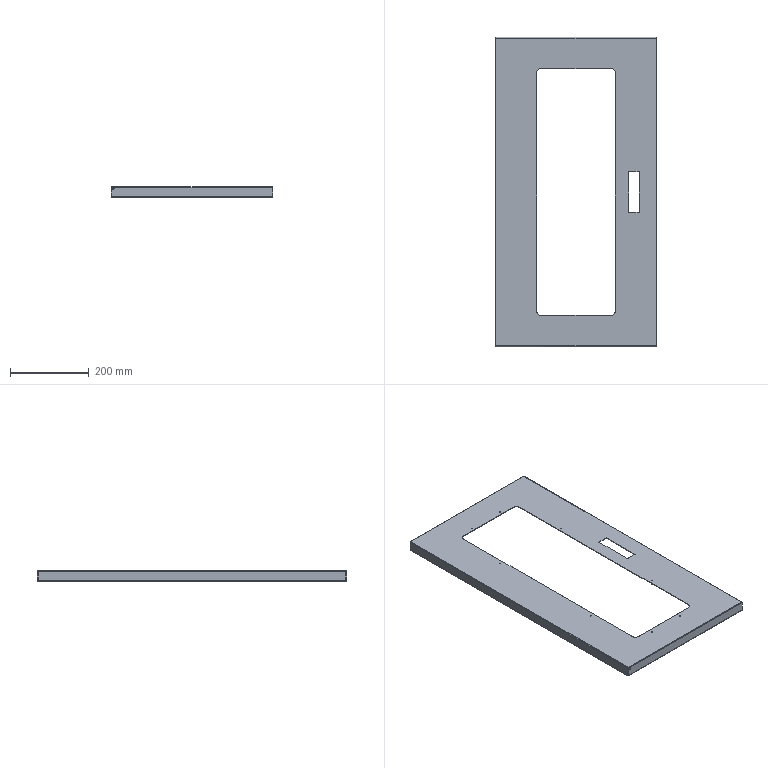Part | SolidWorks | features ICE 4, EdgeFlange 2, MirrorPattern 2, Fillet 1, FlatPattern 1, HoleWzd 1, SMBaseFlange 1, SheetMetal 1 | 1 solid | 110 faces | box 411 x 786 x 26.5 mm | volume 442380 mm3 | plane 54 | cylinder 40 | spline 16 | commonest cylinder face diameters 3 x16 1 x8 4 x8 5 x4 20 x4